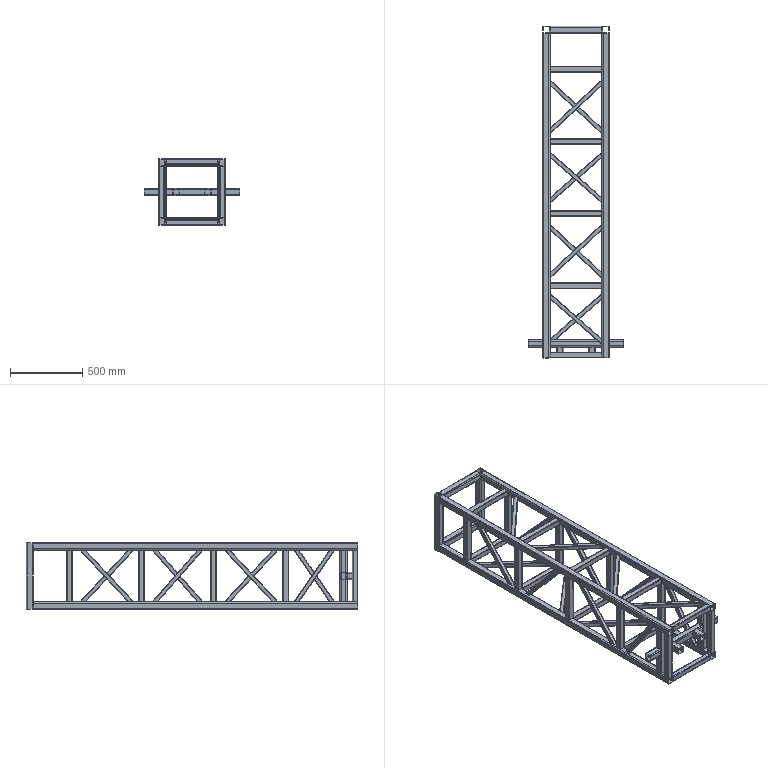Part | SolidWorks | features WeldCornerFeat 8, WeldMemberFeat 7, LPattern 3, CirPattern 2, 3DProfileFeature 1, MirrorSolid 1, RefAxis 1, WeldmentFeature 1 | 51 solids | 918 faces | box 660 x 2300 x 460 mm | volume 12314048 mm3 | plane 510 | cylinder 408 | commonest cylinder face diameters 8 x188 4 x128 16 x60 6 x16 12 x16